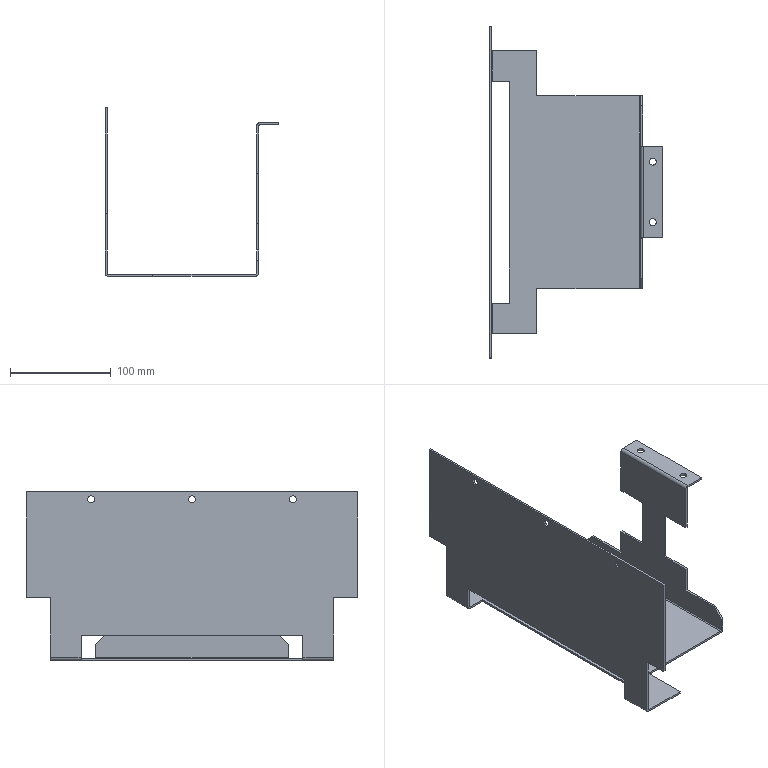Part | STEP file | PN_0022_default | 1 solid | 56 faces | box 172 x 329 x 167 mm | volume 178980 mm3 | plane 38 | cylinder 18 | commonest cylinder face diameters 7 x10 2 x4 6 x4